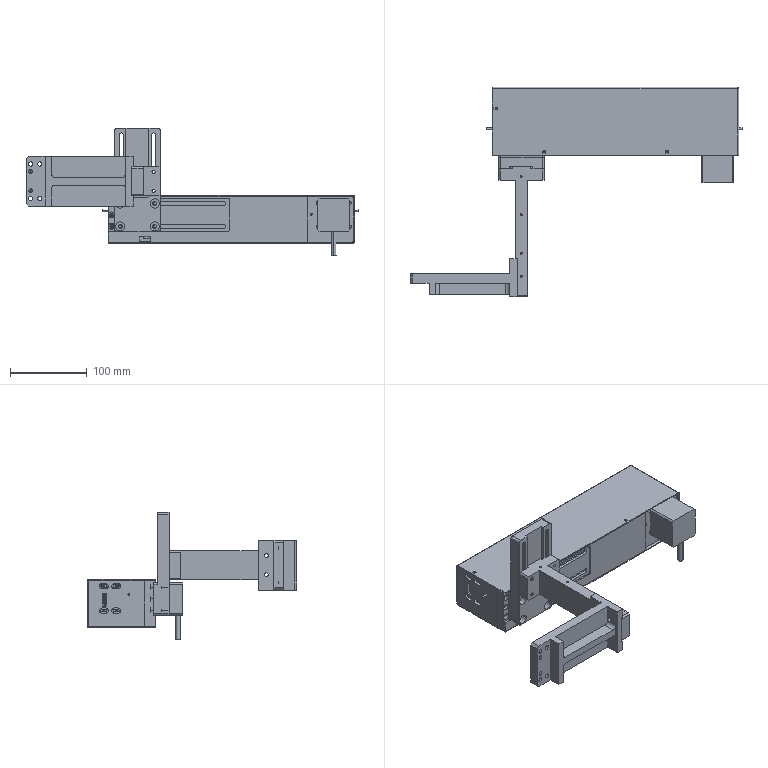Part | NX | features BREP 49 | 60 solids | 3393 faces | volume 931927 mm3 | cylinder 1491 | plane 1095 | cone 309 | sphere 308 | torus 186 | spline 4 | commonest cylinder face diameters 2.5 x211 0.56 x126 0.3 x116 3.95 x112 6 x110 3.4 x88